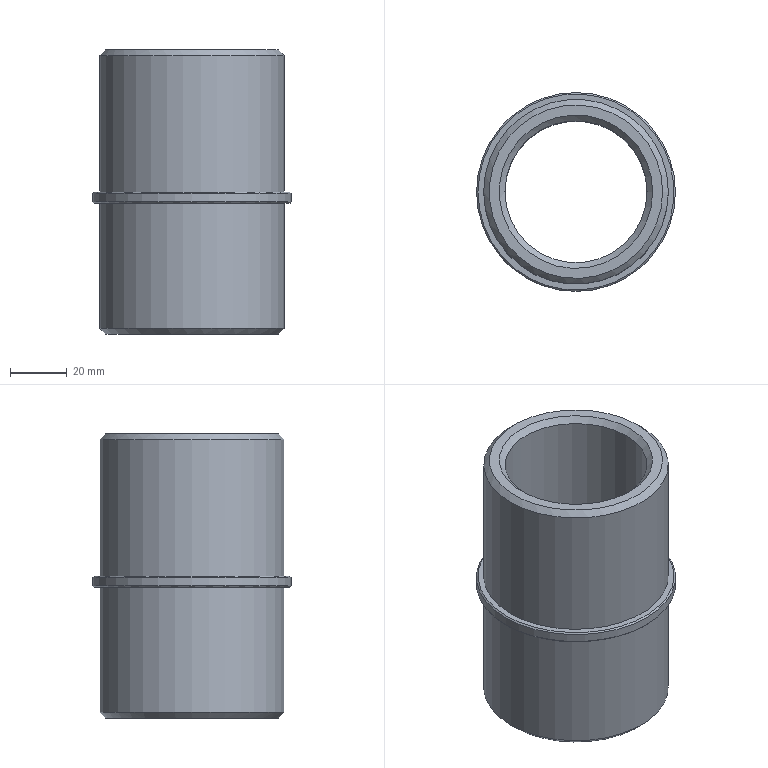Part | STEP file | solid 5 | 1 solid | 14 faces | box 70 x 70 x 100 mm | volume 136102 mm3 | cone 6 | plane 4 | cylinder 4 | commonest cylinder face diameters 65 x2 50 x1 70 x1